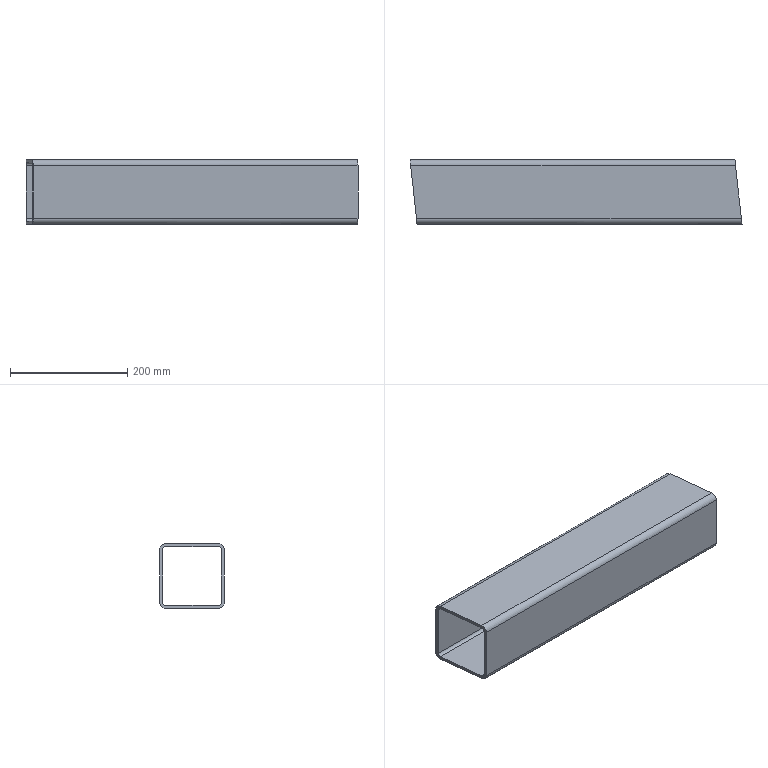Part | SolidWorks | features 3DProfileFeature 1, ICE 1, WeldMemberFeat 1, WeldmentFeature 1 | 1 solid | 18 faces | box 565.469 x 110 x 110 mm | volume 1126381 mm3 | plane 10 | cylinder 8 | commonest cylinder face diameters 10 x4 20 x4
STEP:
#1=CARTESIAN_POINT('',(563.658,55.,-45.));
#2=VERTEX_POINT('',#1);
#3=CARTESIAN_POINT('',(10.323,55.,-45.));
#4=VERTEX_POINT('',#3);
#5=CARTESIAN_POINT('',(600.,55.,-45.));
#6=DIRECTION('',(-1.,0.,0.));
#7=VECTOR('',#6,1000.);
#8=LINE('',#5,#7);
#9=EDGE_CURVE('',#2,#4,#8,.T.);
#10=ORIENTED_EDGE('',*,*,#9,.F.);
#11=CARTESIAN_POINT('',(564.761,45.,-55.));
#12=VERTEX_POINT('',#11);
#13=CARTESIAN_POINT('',(563.658,55.,-45.));
#14=CARTESIAN_POINT('',(563.658,55.,-50.858));
#15=CARTESIAN_POINT('',(564.115,50.858,-55.));
#16=CARTESIAN_POINT('',(564.761,45.,-55.));
#17=(BOUNDED_CURVE()B_SPLINE_CURVE(3,(#13,#14,#15,#16),.UNSPECIFIED.,.F.,.F.)B_SPLINE_CURVE_WITH_KNOTS((4,4),(0.,1.571),.UNSPECIFIED.)CURVE()GEOMETRIC_REPRESENTATION_ITEM()RATIONAL_B_SPLINE_CURVE((1.,0.8047,0.8047,1.))REPRESENTATION_ITEM(''));
#18=EDGE_CURVE('',#2,#12,#17,.T.);
#19=ORIENTED_EDGE('',*,*,#18,.T.);
#20=CARTESIAN_POINT('',(11.426,45.,-55.));
#21=VERTEX_POINT('',#20);
#22=CARTESIAN_POINT('',(600.,45.,-55.));
#23=DIRECTION('',(-1.,0.,0.));
#24=VECTOR('',#23,1000.);
#25=LINE('',#22,#24);
#26=EDGE_CURVE('',#12,#21,#25,.T.);
#27=ORIENTED_EDGE('',*,*,#26,.T.);
#28=CARTESIAN_POINT('',(11.426,45.,-55.));
#29=CARTESIAN_POINT('',(10.779,50.858,-55.));
#30=CARTESIAN_POINT('',(10.323,55.,-50.858));
#31=CARTESIAN_POINT('',(10.323,55.,-45.));
#32=(BOUNDED_CURVE()B_SPLINE_CURVE(3,(#28,#29,#30,#31),.UNSPECIFIED.,.F.,.F.)B_SPLINE_CURVE_WITH_KNOTS((4,4),(4.712,6.283),.UNSPECIFIED.)CURVE()GEOMETRIC_REPRESENTATION_ITEM()RATIONAL_B_SPLINE_CURVE((1.,0.8047,0.8047,1.))REPRESENTATION_ITEM(''));
#33=EDGE_CURVE('',#21,#4,#32,.T.);
#34=ORIENTED_EDGE('',*,*,#33,.T.);
#35=EDGE_LOOP('',(#10,#19,#27,#34));
#36=FACE_OUTER_BOUND('',#35,.T.);
#37=CARTESIAN_POINT('',(600.,45.,-45.));
#38=DIRECTION('',(-1.,0.,0.));
#39=DIRECTION('',(0.,0.,1.));
#40=AXIS2_PLACEMENT_3D('',#37,#38,#39);
#41=CYLINDRICAL_SURFACE('',#40,10.);
#42=ADVANCED_FACE('',(#36),#41,.T.);
#43=CARTESIAN_POINT('',(563.658,55.,45.));
#44=VERTEX_POINT('',#43);
#45=CARTESIAN_POINT('',(10.323,55.,45.));
#46=VERTEX_POINT('',#45);
#47=CARTESIAN_POINT('',(600.,55.,45.));
#48=DIRECTION('',(-1.,0.,0.));
#49=VECTOR('',#48,1000.);
#50=LINE('',#47,#49);
#51=EDGE_CURVE('',#44,#46,#50,.T.);
#52=ORIENTED_EDGE('',*,*,#51,.F.);
#53=CARTESIAN_POINT('',(563.658,55.,-386.466));
#54=DIRECTION('',(0.,0.,1.));
#55=VECTOR('',#54,1000.);
#56=LINE('',#53,#55);
#57=EDGE_CURVE('',#2,#44,#56,.T.);
#58=ORIENTED_EDGE('',*,*,#57,.F.);
#59=ORIENTED_EDGE('',*,*,#9,.T.);
#60=CARTESIAN_POINT('',(10.323,55.,-45.));
#61=DIRECTION('',(0.,0.,1.));
#62=VECTOR('',#61,1000.);
#63=LINE('',#60,#62);
#64=EDGE_CURVE('',#4,#46,#63,.T.);
#65=ORIENTED_EDGE('',*,*,#64,.T.);
#66=EDGE_LOOP('',(#52,#58,#59,#65));
#67=FACE_OUTER_BOUND('',#66,.T.);
#68=CARTESIAN_POINT('',(600.,55.,-45.));
#69=DIRECTION('',(0.,-1.,0.));
#70=DIRECTION('',(0.,0.,-1.));
#71=AXIS2_PLACEMENT_3D('',#68,#69,#70);
#72=PLANE('',#71);
#73=ADVANCED_FACE('',(#67),#72,.F.);
#74=CARTESIAN_POINT('',(564.761,45.,55.));
#75=VERTEX_POINT('',#74);
#76=CARTESIAN_POINT('',(11.426,45.,55.));
#77=VERTEX_POINT('',#76);
#78=CARTESIAN_POINT('',(600.,45.,55.));
#79=DIRECTION('',(-1.,0.,0.));
#80=VECTOR('',#79,1000.);
#81=LINE('',#78,#80);
#82=EDGE_CURVE('',#75,#77,#81,.T.);
#83=ORIENTED_EDGE('',*,*,#82,.F.);
#84=CARTESIAN_POINT('',(564.761,45.,55.));
#85=CARTESIAN_POINT('',(564.115,50.858,55.));
#86=CARTESIAN_POINT('',(563.658,55.,50.858));
#87=CARTESIAN_POINT('',(563.658,55.,45.));
#88=(BOUNDED_CURVE()B_SPLINE_CURVE(3,(#84,#85,#86,#87),.UNSPECIFIED.,.F.,.F.)B_SPLINE_CURVE_WITH_KNOTS((4,4),(4.712,6.283),.UNSPECIFIED.)CURVE()GEOMETRIC_REPRESENTATION_ITEM()RATIONAL_B_SPLINE_CURVE((1.,0.8047,0.8047,1.))REPRESENTATION_ITEM(''));
#89=EDGE_CURVE('',#75,#44,#88,.T.);
#90=ORIENTED_EDGE('',*,*,#89,.T.);
#91=ORIENTED_EDGE('',*,*,#51,.T.);
#92=CARTESIAN_POINT('',(10.323,55.,45.));
#93=CARTESIAN_POINT('',(10.323,55.,50.858));
#94=CARTESIAN_POINT('',(10.779,50.858,55.));
#95=CARTESIAN_POINT('',(11.426,45.,55.));
#96=(BOUNDED_CURVE()B_SPLINE_CURVE(3,(#92,#93,#94,#95),.UNSPECIFIED.,.F.,.F.)B_SPLINE_CURVE_WITH_KNOTS((4,4),(0.,1.571),.UNSPECIFIED.)CURVE()GEOMETRIC_REPRESENTATION_ITEM()RATIONAL_B_SPLINE_CURVE((1.,0.8047,0.8047,1.))REPRESENTATION_ITEM(''));
#97=EDGE_CURVE('',#46,#77,#96,.T.);
#98=ORIENTED_EDGE('',*,*,#97,.T.);
#99=EDGE_LOOP('',(#83,#90,#91,#98));
#100=FACE_OUTER_BOUND('',#99,.T.);
#101=CARTESIAN_POINT('',(600.,45.,45.));
#102=DIRECTION('',(-1.,0.,0.));
#103=DIRECTION('',(0.,0.,1.));
#104=AXIS2_PLACEMENT_3D('',#101,#102,#103);
#105=CYLINDRICAL_SURFACE('',#104,10.);
#106=ADVANCED_FACE('',(#100),#105,.T.);
#107=CARTESIAN_POINT('',(574.689,-45.,55.));
#108=VERTEX_POINT('',#107);
#109=CARTESIAN_POINT('',(21.353,-45.,55.));
#110=VERTEX_POINT('',#109);
#111=CARTESIAN_POINT('',(600.,-45.,55.));
#112=DIRECTION('',(-1.,0.,0.));
#113=VECTOR('',#112,1000.);
#114=LINE('',#111,#113);
#115=EDGE_CURVE('',#108,#110,#114,.T.);
#116=ORIENTED_EDGE('',*,*,#115,.F.);
#117=CARTESIAN_POINT('',(600.,-274.468,55.));
#118=DIRECTION('',(0.1096,-0.994,0.));
#119=VECTOR('',#118,1000.);
#120=LINE('',#117,#119);
#121=EDGE_CURVE('',#75,#108,#120,.T.);
#122=ORIENTED_EDGE('',*,*,#121,.F.);
#123=ORIENTED_EDGE('',*,*,#82,.T.);
#124=CARTESIAN_POINT('',(0.,148.583,55.));
#125=DIRECTION('',(-0.1096,0.994,0.));
#126=VECTOR('',#125,1000.);
#127=LINE('',#124,#126);
#128=EDGE_CURVE('',#110,#77,#127,.T.);
#129=ORIENTED_EDGE('',*,*,#128,.F.);
#130=EDGE_LOOP('',(#116,#122,#123,#129));
#131=FACE_OUTER_BOUND('',#130,.T.);
#132=CARTESIAN_POINT('',(600.,-45.,55.));
#133=DIRECTION('',(0.,0.,-1.));
#134=DIRECTION('',(-1.,0.,0.));
#135=AXIS2_PLACEMENT_3D('',#132,#133,#134);
#136=PLANE('',#135);
#137=ADVANCED_FACE('',(#131),#136,.F.);
#138=CARTESIAN_POINT('',(575.792,-55.,45.));
#139=VERTEX_POINT('',#138);
#140=CARTESIAN_POINT('',(22.456,-55.,45.));
#141=VERTEX_POINT('',#140);
#142=CARTESIAN_POINT('',(600.,-55.,45.));
#143=DIRECTION('',(-1.,0.,0.));
#144=VECTOR('',#143,1000.);
#145=LINE('',#142,#144);
#146=EDGE_CURVE('',#139,#141,#145,.T.);
#147=ORIENTED_EDGE('',*,*,#146,.F.);
#148=CARTESIAN_POINT('',(575.792,-55.,45.));
#149=CARTESIAN_POINT('',(575.792,-55.,50.858));
#150=CARTESIAN_POINT('',(575.335,-50.858,55.));
#151=CARTESIAN_POINT('',(574.689,-45.,55.));
#152=(BOUNDED_CURVE()B_SPLINE_CURVE(3,(#148,#149,#150,#151),.UNSPECIFIED.,.F.,.F.)B_SPLINE_CURVE_WITH_KNOTS((4,4),(3.142,4.712),.UNSPECIFIED.)CURVE()GEOMETRIC_REPRESENTATION_ITEM()RATIONAL_B_SPLINE_CURVE((1.,0.8047,0.8047,1.))REPRESENTATION_ITEM(''));
#153=EDGE_CURVE('',#139,#108,#152,.T.);
#154=ORIENTED_EDGE('',*,*,#153,.T.);
#155=ORIENTED_EDGE('',*,*,#115,.T.);
#156=CARTESIAN_POINT('',(21.353,-45.,55.));
#157=CARTESIAN_POINT('',(21.999,-50.858,55.));
#158=CARTESIAN_POINT('',(22.456,-55.,50.858));
#159=CARTESIAN_POINT('',(22.456,-55.,45.));
#160=(BOUNDED_CURVE()B_SPLINE_CURVE(3,(#156,#157,#158,#159),.UNSPECIFIED.,.F.,.F.)B_SPLINE_CURVE_WITH_KNOTS((4,4),(1.571,3.142),.UNSPECIFIED.)CURVE()GEOMETRIC_REPRESENTATION_ITEM()RATIONAL_B_SPLINE_CURVE((1.,0.8047,0.8047,1.))REPRESENTATION_ITEM(''));
#161=EDGE_CURVE('',#110,#141,#160,.T.);
#162=ORIENTED_EDGE('',*,*,#161,.T.);
#163=EDGE_LOOP('',(#147,#154,#155,#162));
#164=FACE_OUTER_BOUND('',#163,.T.);
#165=CARTESIAN_POINT('',(600.,-45.,45.));
#166=DIRECTION('',(-1.,0.,0.));
#167=DIRECTION('',(0.,0.,1.));
#168=AXIS2_PLACEMENT_3D('',#165,#166,#167);
#169=CYLINDRICAL_SURFACE('',#168,10.);
#170=ADVANCED_FACE('',(#164),#169,.T.);
#171=CARTESIAN_POINT('',(575.792,-55.,-45.));
#172=VERTEX_POINT('',#171);
#173=CARTESIAN_POINT('',(22.456,-55.,-45.));
#174=VERTEX_POINT('',#173);
#175=CARTESIAN_POINT('',(600.,-55.,-45.));
#176=DIRECTION('',(-1.,0.,0.));
#177=VECTOR('',#176,1000.);
#178=LINE('',#175,#177);
#179=EDGE_CURVE('',#172,#174,#178,.T.);
#180=ORIENTED_EDGE('',*,*,#179,.F.);
#181=CARTESIAN_POINT('',(575.792,-55.,45.));
#182=DIRECTION('',(0.,0.,1.));
#183=VECTOR('',#182,1000.);
#184=LINE('',#181,#183);
#185=EDGE_CURVE('',#172,#139,#184,.T.);
#186=ORIENTED_EDGE('',*,*,#185,.T.);
#187=ORIENTED_EDGE('',*,*,#146,.T.);
#188=CARTESIAN_POINT('',(22.456,-55.,-386.466));
#189=DIRECTION('',(0.,0.,1.));
#190=VECTOR('',#189,1000.);
#191=LINE('',#188,#190);
#192=EDGE_CURVE('',#174,#141,#191,.T.);
#193=ORIENTED_EDGE('',*,*,#192,.F.);
#194=EDGE_LOOP('',(#180,#186,#187,#193));
#195=FACE_OUTER_BOUND('',#194,.T.);
#196=CARTESIAN_POINT('',(600.,-55.,45.));
#197=DIRECTION('',(0.,1.,0.));
#198=DIRECTION('',(0.,0.,1.));
#199=AXIS2_PLACEMENT_3D('',#196,#197,#198);
#200=PLANE('',#199);
#201=ADVANCED_FACE('',(#195),#200,.F.);
#202=CARTESIAN_POINT('',(574.689,-45.,-55.));
#203=VERTEX_POINT('',#202);
#204=CARTESIAN_POINT('',(21.353,-45.,-55.));
#205=VERTEX_POINT('',#204);
#206=CARTESIAN_POINT('',(600.,-45.,-55.));
#207=DIRECTION('',(-1.,0.,0.));
#208=VECTOR('',#207,1000.);
#209=LINE('',#206,#208);
#210=EDGE_CURVE('',#203,#205,#209,.T.);
#211=ORIENTED_EDGE('',*,*,#210,.F.);
#212=CARTESIAN_POINT('',(574.689,-45.,-55.));
#213=CARTESIAN_POINT('',(575.335,-50.858,-55.));
#214=CARTESIAN_POINT('',(575.792,-55.,-50.858));
#215=CARTESIAN_POINT('',(575.792,-55.,-45.));
#216=(BOUNDED_CURVE()B_SPLINE_CURVE(3,(#212,#213,#214,#215),.UNSPECIFIED.,.F.,.F.)B_SPLINE_CURVE_WITH_KNOTS((4,4),(1.571,3.142),.UNSPECIFIED.)CURVE()GEOMETRIC_REPRESENTATION_ITEM()RATIONAL_B_SPLINE_CURVE((1.,0.8047,0.8047,1.))REPRESENTATION_ITEM(''));
#217=EDGE_CURVE('',#203,#172,#216,.T.);
#218=ORIENTED_EDGE('',*,*,#217,.T.);
#219=ORIENTED_EDGE('',*,*,#179,.T.);
#220=CARTESIAN_POINT('',(22.456,-55.,-45.));
#221=CARTESIAN_POINT('',(22.456,-55.,-50.858));
#222=CARTESIAN_POINT('',(21.999,-50.858,-55.));
#223=CARTESIAN_POINT('',(21.353,-45.,-55.));
#224=(BOUNDED_CURVE()B_SPLINE_CURVE(3,(#220,#221,#222,#223),.UNSPECIFIED.,.F.,.F.)B_SPLINE_CURVE_WITH_KNOTS((4,4),(3.142,4.712),.UNSPECIFIED.)CURVE()GEOMETRIC_REPRESENTATION_ITEM()RATIONAL_B_SPLINE_CURVE((1.,0.8047,0.8047,1.))REPRESENTATION_ITEM(''));
#225=EDGE_CURVE('',#174,#205,#224,.T.);
#226=ORIENTED_EDGE('',*,*,#225,.T.);
#227=EDGE_LOOP('',(#211,#218,#219,#226));
#228=FACE_OUTER_BOUND('',#227,.T.);
#229=CARTESIAN_POINT('',(600.,-45.,-45.));
#230=DIRECTION('',(-1.,0.,0.));
#231=DIRECTION('',(0.,0.,1.));
#232=AXIS2_PLACEMENT_3D('',#229,#230,#231);
#233=CYLINDRICAL_SURFACE('',#232,10.);
#234=ADVANCED_FACE('',(#228),#233,.T.);
#235=CARTESIAN_POINT('',(564.761,45.,50.));
#236=VERTEX_POINT('',#235);
#237=CARTESIAN_POINT('',(564.21,50.,45.));
#238=VERTEX_POINT('',#237);
#239=CARTESIAN_POINT('',(564.761,45.,50.));
#240=CARTESIAN_POINT('',(564.438,47.929,50.));
#241=CARTESIAN_POINT('',(564.21,50.,47.929));
#242=CARTESIAN_POINT('',(564.21,50.,45.));
#243=(BOUNDED_CURVE()B_SPLINE_CURVE(3,(#239,#240,#241,#242),.UNSPECIFIED.,.F.,.F.)B_SPLINE_CURVE_WITH_KNOTS((4,4),(4.712,6.283),.UNSPECIFIED.)CURVE()GEOMETRIC_REPRESENTATION_ITEM()RATIONAL_B_SPLINE_CURVE((1.,0.8047,0.8047,1.))REPRESENTATION_ITEM(''));
#244=EDGE_CURVE('',#236,#238,#243,.T.);
#245=ORIENTED_EDGE('',*,*,#244,.F.);
#246=CARTESIAN_POINT('',(11.426,45.,50.));
#247=VERTEX_POINT('',#246);
#248=CARTESIAN_POINT('',(600.,45.,50.));
#249=DIRECTION('',(-1.,0.,0.));
#250=VECTOR('',#249,1000.);
#251=LINE('',#248,#250);
#252=EDGE_CURVE('',#236,#247,#251,.T.);
#253=ORIENTED_EDGE('',*,*,#252,.T.);
#254=CARTESIAN_POINT('',(10.874,50.,45.));
#255=VERTEX_POINT('',#254);
#256=CARTESIAN_POINT('',(10.874,50.,45.));
#257=CARTESIAN_POINT('',(10.874,50.,47.929));
#258=CARTESIAN_POINT('',(11.103,47.929,50.));
#259=CARTESIAN_POINT('',(11.426,45.,50.));
#260=(BOUNDED_CURVE()B_SPLINE_CURVE(3,(#256,#257,#258,#259),.UNSPECIFIED.,.F.,.F.)B_SPLINE_CURVE_WITH_KNOTS((4,4),(0.,1.571),.UNSPECIFIED.)CURVE()GEOMETRIC_REPRESENTATION_ITEM()RATIONAL_B_SPLINE_CURVE((1.,0.8047,0.8047,1.))REPRESENTATION_ITEM(''));
#261=EDGE_CURVE('',#255,#247,#260,.T.);
#262=ORIENTED_EDGE('',*,*,#261,.F.);
#263=CARTESIAN_POINT('',(600.,50.,45.));
#264=DIRECTION('',(-1.,0.,0.));
#265=VECTOR('',#264,1000.);
#266=LINE('',#263,#265);
#267=EDGE_CURVE('',#238,#255,#266,.T.);
#268=ORIENTED_EDGE('',*,*,#267,.F.);
#269=EDGE_LOOP('',(#245,#253,#262,#268));
#270=FACE_OUTER_BOUND('',#269,.T.);
#271=CARTESIAN_POINT('',(600.,45.,45.));
#272=DIRECTION('',(-1.,0.,0.));
#273=DIRECTION('',(0.,0.,1.));
#274=AXIS2_PLACEMENT_3D('',#271,#272,#273);
#275=CYLINDRICAL_SURFACE('',#274,5.);
#276=ADVANCED_FACE('',(#270),#275,.F.);
#277=CARTESIAN_POINT('',(564.21,50.,-45.));
#278=VERTEX_POINT('',#277);
#279=CARTESIAN_POINT('',(564.21,50.,-45.));
#280=DIRECTION('',(0.,0.,-1.));
#281=VECTOR('',#280,1000.);
#282=LINE('',#279,#281);
#283=EDGE_CURVE('',#238,#278,#282,.T.);
#284=ORIENTED_EDGE('',*,*,#283,.F.);
#285=ORIENTED_EDGE('',*,*,#267,.T.);
#286=CARTESIAN_POINT('',(10.874,50.,-45.));
#287=VERTEX_POINT('',#286);
#288=CARTESIAN_POINT('',(10.874,50.,-45.));
#289=DIRECTION('',(0.,0.,1.));
#290=VECTOR('',#289,1000.);
#291=LINE('',#288,#290);
#292=EDGE_CURVE('',#287,#255,#291,.T.);
#293=ORIENTED_EDGE('',*,*,#292,.F.);
#294=CARTESIAN_POINT('',(600.,50.,-45.));
#295=DIRECTION('',(-1.,0.,0.));
#296=VECTOR('',#295,1000.);
#297=LINE('',#294,#296);
#298=EDGE_CURVE('',#278,#287,#297,.T.);
#299=ORIENTED_EDGE('',*,*,#298,.F.);
#300=EDGE_LOOP('',(#284,#285,#293,#299));
#301=FACE_OUTER_BOUND('',#300,.T.);
#302=CARTESIAN_POINT('',(600.,50.,-45.));
#303=DIRECTION('',(0.,-1.,0.));
#304=DIRECTION('',(0.,0.,-1.));
#305=AXIS2_PLACEMENT_3D('',#302,#303,#304);
#306=PLANE('',#305);
#307=ADVANCED_FACE('',(#301),#306,.T.);
#308=CARTESIAN_POINT('',(564.761,45.,-50.));
#309=VERTEX_POINT('',#308);
#310=CARTESIAN_POINT('',(564.21,50.,-45.));
#311=CARTESIAN_POINT('',(564.21,50.,-47.929));
#312=CARTESIAN_POINT('',(564.438,47.929,-50.));
#313=CARTESIAN_POINT('',(564.761,45.,-50.));
#314=(BOUNDED_CURVE()B_SPLINE_CURVE(3,(#310,#311,#312,#313),.UNSPECIFIED.,.F.,.F.)B_SPLINE_CURVE_WITH_KNOTS((4,4),(0.,1.571),.UNSPECIFIED.)CURVE()GEOMETRIC_REPRESENTATION_ITEM()RATIONAL_B_SPLINE_CURVE((1.,0.8047,0.8047,1.))REPRESENTATION_ITEM(''));
#315=EDGE_CURVE('',#278,#309,#314,.T.);
#316=ORIENTED_EDGE('',*,*,#315,.F.);
#317=ORIENTED_EDGE('',*,*,#298,.T.);
#318=CARTESIAN_POINT('',(11.426,45.,-50.));
#319=VERTEX_POINT('',#318);
#320=CARTESIAN_POINT('',(11.426,45.,-50.));
#321=CARTESIAN_POINT('',(11.103,47.929,-50.));
#322=CARTESIAN_POINT('',(10.874,50.,-47.929));
#323=CARTESIAN_POINT('',(10.874,50.,-45.));
#324=(BOUNDED_CURVE()B_SPLINE_CURVE(3,(#320,#321,#322,#323),.UNSPECIFIED.,.F.,.F.)B_SPLINE_CURVE_WITH_KNOTS((4,4),(4.712,6.283),.UNSPECIFIED.)CURVE()GEOMETRIC_REPRESENTATION_ITEM()RATIONAL_B_SPLINE_CURVE((1.,0.8047,0.8047,1.))REPRESENTATION_ITEM(''));
#325=EDGE_CURVE('',#319,#287,#324,.T.);
#326=ORIENTED_EDGE('',*,*,#325,.F.);
#327=CARTESIAN_POINT('',(600.,45.,-50.));
#328=DIRECTION('',(-1.,0.,0.));
#329=VECTOR('',#328,1000.);
#330=LINE('',#327,#329);
#331=EDGE_CURVE('',#309,#319,#330,.T.);
#332=ORIENTED_EDGE('',*,*,#331,.F.);
#333=EDGE_LOOP('',(#316,#317,#326,#332));
#334=FACE_OUTER_BOUND('',#333,.T.);
#335=CARTESIAN_POINT('',(600.,45.,-45.));
#336=DIRECTION('',(-1.,0.,0.));
#337=DIRECTION('',(0.,0.,1.));
#338=AXIS2_PLACEMENT_3D('',#335,#336,#337);
#339=CYLINDRICAL_SURFACE('',#338,5.);
#340=ADVANCED_FACE('',(#334),#339,.F.);
#341=CARTESIAN_POINT('',(574.689,-45.,-50.));
#342=VERTEX_POINT('',#341);
#343=CARTESIAN_POINT('',(565.185,41.16,-50.));
#344=DIRECTION('',(0.1096,-0.994,0.));
#345=VECTOR('',#344,1000.);
#346=LINE('',#343,#345);
#347=EDGE_CURVE('',#309,#342,#346,.T.);
#348=ORIENTED_EDGE('',*,*,#347,.F.);
#349=ORIENTED_EDGE('',*,*,#331,.T.);
#350=CARTESIAN_POINT('',(21.353,-45.,-50.));
#351=VERTEX_POINT('',#350);
#352=CARTESIAN_POINT('',(18.501,-19.142,-50.));
#353=DIRECTION('',(-0.1096,0.994,0.));
#354=VECTOR('',#353,1000.);
#355=LINE('',#352,#354);
#356=EDGE_CURVE('',#351,#319,#355,.T.);
#357=ORIENTED_EDGE('',*,*,#356,.F.);
#358=CARTESIAN_POINT('',(600.,-45.,-50.));
#359=DIRECTION('',(-1.,0.,0.));
#360=VECTOR('',#359,1000.);
#361=LINE('',#358,#360);
#362=EDGE_CURVE('',#342,#351,#361,.T.);
#363=ORIENTED_EDGE('',*,*,#362,.F.);
#364=EDGE_LOOP('',(#348,#349,#357,#363));
#365=FACE_OUTER_BOUND('',#364,.T.);
#366=CARTESIAN_POINT('',(600.,45.,-50.));
#367=DIRECTION('',(0.,0.,1.));
#368=DIRECTION('',(1.,0.,0.));
#369=AXIS2_PLACEMENT_3D('',#366,#367,#368);
#370=PLANE('',#369);
#371=ADVANCED_FACE('',(#365),#370,.T.);
#372=CARTESIAN_POINT('',(575.24,-50.,-45.));
#373=VERTEX_POINT('',#372);
#374=CARTESIAN_POINT('',(574.689,-45.,-50.));
#375=CARTESIAN_POINT('',(575.012,-47.929,-50.));
#376=CARTESIAN_POINT('',(575.24,-50.,-47.929));
#377=CARTESIAN_POINT('',(575.24,-50.,-45.));
#378=(BOUNDED_CURVE()B_SPLINE_CURVE(3,(#374,#375,#376,#377),.UNSPECIFIED.,.F.,.F.)B_SPLINE_CURVE_WITH_KNOTS((4,4),(1.571,3.142),.UNSPECIFIED.)CURVE()GEOMETRIC_REPRESENTATION_ITEM()RATIONAL_B_SPLINE_CURVE((1.,0.8047,0.8047,1.))REPRESENTATION_ITEM(''));
#379=EDGE_CURVE('',#342,#373,#378,.T.);
#380=ORIENTED_EDGE('',*,*,#379,.F.);
#381=ORIENTED_EDGE('',*,*,#362,.T.);
#382=CARTESIAN_POINT('',(21.904,-50.,-45.));
#383=VERTEX_POINT('',#382);
#384=CARTESIAN_POINT('',(21.904,-50.,-45.));
#385=CARTESIAN_POINT('',(21.904,-50.,-47.929));
#386=CARTESIAN_POINT('',(21.676,-47.929,-50.));
#387=CARTESIAN_POINT('',(21.353,-45.,-50.));
#388=(BOUNDED_CURVE()B_SPLINE_CURVE(3,(#384,#385,#386,#387),.UNSPECIFIED.,.F.,.F.)B_SPLINE_CURVE_WITH_KNOTS((4,4),(3.142,4.712),.UNSPECIFIED.)CURVE()GEOMETRIC_REPRESENTATION_ITEM()RATIONAL_B_SPLINE_CURVE((1.,0.8047,0.8047,1.))REPRESENTATION_ITEM(''));
#389=EDGE_CURVE('',#383,#351,#388,.T.);
#390=ORIENTED_EDGE('',*,*,#389,.F.);
#391=CARTESIAN_POINT('',(600.,-50.,-45.));
#392=DIRECTION('',(-1.,0.,0.));
#393=VECTOR('',#392,1000.);
#394=LINE('',#391,#393);
#395=EDGE_CURVE('',#373,#383,#394,.T.);
#396=ORIENTED_EDGE('',*,*,#395,.F.);
#397=EDGE_LOOP('',(#380,#381,#390,#396));
#398=FACE_OUTER_BOUND('',#397,.T.);
#399=CARTESIAN_POINT('',(600.,-45.,-45.));
#400=DIRECTION('',(-1.,0.,0.));
#401=DIRECTION('',(0.,0.,1.));
#402=AXIS2_PLACEMENT_3D('',#399,#400,#401);
#403=CYLINDRICAL_SURFACE('',#402,5.);
#404=ADVANCED_FACE('',(#398),#403,.F.);
#405=CARTESIAN_POINT('',(575.24,-50.,45.));
#406=VERTEX_POINT('',#405);
#407=CARTESIAN_POINT('',(575.24,-50.,45.));
#408=DIRECTION('',(0.,0.,1.));
#409=VECTOR('',#408,1000.);
#410=LINE('',#407,#409);
#411=EDGE_CURVE('',#373,#406,#410,.T.);
#412=ORIENTED_EDGE('',*,*,#411,.F.);
#413=ORIENTED_EDGE('',*,*,#395,.T.);
#414=CARTESIAN_POINT('',(21.904,-50.,45.));
#415=VERTEX_POINT('',#414);
#416=CARTESIAN_POINT('',(21.904,-50.,45.));
#417=DIRECTION('',(0.,0.,-1.));
#418=VECTOR('',#417,1000.);
#419=LINE('',#416,#418);
#420=EDGE_CURVE('',#415,#383,#419,.T.);
#421=ORIENTED_EDGE('',*,*,#420,.F.);
#422=CARTESIAN_POINT('',(600.,-50.,45.));
#423=DIRECTION('',(-1.,0.,0.));
#424=VECTOR('',#423,1000.);
#425=LINE('',#422,#424);
#426=EDGE_CURVE('',#406,#415,#425,.T.);
#427=ORIENTED_EDGE('',*,*,#426,.F.);
#428=EDGE_LOOP('',(#412,#413,#421,#427));
#429=FACE_OUTER_BOUND('',#428,.T.);
#430=CARTESIAN_POINT('',(600.,-50.,45.));
#431=DIRECTION('',(0.,1.,0.));
#432=DIRECTION('',(0.,0.,1.));
#433=AXIS2_PLACEMENT_3D('',#430,#431,#432);
#434=PLANE('',#433);
#435=ADVANCED_FACE('',(#429),#434,.T.);
#436=CARTESIAN_POINT('',(574.689,-45.,50.));
#437=VERTEX_POINT('',#436);
#438=CARTESIAN_POINT('',(575.24,-50.,45.));
#439=CARTESIAN_POINT('',(575.24,-50.,47.929));
#440=CARTESIAN_POINT('',(575.012,-47.929,50.));
#441=CARTESIAN_POINT('',(574.689,-45.,50.));
#442=(BOUNDED_CURVE()B_SPLINE_CURVE(3,(#438,#439,#440,#441),.UNSPECIFIED.,.F.,.F.)B_SPLINE_CURVE_WITH_KNOTS((4,4),(3.142,4.712),.UNSPECIFIED.)CURVE()GEOMETRIC_REPRESENTATION_ITEM()RATIONAL_B_SPLINE_CURVE((1.,0.8047,0.8047,1.))REPRESENTATION_ITEM(''));
#443=EDGE_CURVE('',#406,#437,#442,.T.);
#444=ORIENTED_EDGE('',*,*,#443,.F.);
#445=ORIENTED_EDGE('',*,*,#426,.T.);
#446=CARTESIAN_POINT('',(21.353,-45.,50.));
#447=VERTEX_POINT('',#446);
#448=CARTESIAN_POINT('',(21.353,-45.,50.));
#449=CARTESIAN_POINT('',(21.676,-47.929,50.));
#450=CARTESIAN_POINT('',(21.904,-50.,47.929));
#451=CARTESIAN_POINT('',(21.904,-50.,45.));
#452=(BOUNDED_CURVE()B_SPLINE_CURVE(3,(#448,#449,#450,#451),.UNSPECIFIED.,.F.,.F.)B_SPLINE_CURVE_WITH_KNOTS((4,4),(1.571,3.142),.UNSPECIFIED.)CURVE()GEOMETRIC_REPRESENTATION_ITEM()RATIONAL_B_SPLINE_CURVE((1.,0.8047,0.8047,1.))REPRESENTATION_ITEM(''));
#453=EDGE_CURVE('',#447,#415,#452,.T.);
#454=ORIENTED_EDGE('',*,*,#453,.F.);
#455=CARTESIAN_POINT('',(600.,-45.,50.));
#456=DIRECTION('',(-1.,0.,0.));
#457=VECTOR('',#456,1000.);
#458=LINE('',#455,#457);
#459=EDGE_CURVE('',#437,#447,#458,.T.);
#460=ORIENTED_EDGE('',*,*,#459,.F.);
#461=EDGE_LOOP('',(#444,#445,#454,#460));
#462=FACE_OUTER_BOUND('',#461,.T.);
#463=CARTESIAN_POINT('',(600.,-45.,45.));
#464=DIRECTION('',(-1.,0.,0.));
#465=DIRECTION('',(0.,0.,1.));
#466=AXIS2_PLACEMENT_3D('',#463,#464,#465);
#467=CYLINDRICAL_SURFACE('',#466,5.);
#468=ADVANCED_FACE('',(#462),#467,.F.);
#469=CARTESIAN_POINT('',(574.993,-47.758,50.));
#470=DIRECTION('',(-0.1096,0.994,0.));
#471=VECTOR('',#470,1000.);
#472=LINE('',#469,#471);
#473=EDGE_CURVE('',#437,#236,#472,.T.);
#474=ORIENTED_EDGE('',*,*,#473,.F.);
#475=ORIENTED_EDGE('',*,*,#459,.T.);
#476=CARTESIAN_POINT('',(28.309,-108.06,50.));
#477=DIRECTION('',(0.1096,-0.994,0.));
#478=VECTOR('',#477,1000.);
#479=LINE('',#476,#478);
#480=EDGE_CURVE('',#247,#447,#479,.T.);
#481=ORIENTED_EDGE('',*,*,#480,.F.);
#482=ORIENTED_EDGE('',*,*,#252,.F.);
#483=EDGE_LOOP('',(#474,#475,#481,#482));
#484=FACE_OUTER_BOUND('',#483,.T.);
#485=CARTESIAN_POINT('',(600.,-45.,50.));
#486=DIRECTION('',(0.,0.,-1.));
#487=DIRECTION('',(-1.,0.,0.));
#488=AXIS2_PLACEMENT_3D('',#485,#486,#487);
#489=PLANE('',#488);
#490=ADVANCED_FACE('',(#484),#489,.T.);
#491=ORIENTED_EDGE('',*,*,#26,.F.);
#492=CARTESIAN_POINT('',(600.,-274.468,-55.));
#493=DIRECTION('',(-0.1096,0.994,0.));
#494=VECTOR('',#493,1000.);
#495=LINE('',#492,#494);
#496=EDGE_CURVE('',#203,#12,#495,.T.);
#497=ORIENTED_EDGE('',*,*,#496,.F.);
#498=ORIENTED_EDGE('',*,*,#210,.T.);
#499=CARTESIAN_POINT('',(0.,148.583,-55.));
#500=DIRECTION('',(0.1096,-0.994,0.));
#501=VECTOR('',#500,1000.);
#502=LINE('',#499,#501);
#503=EDGE_CURVE('',#21,#205,#502,.T.);
#504=ORIENTED_EDGE('',*,*,#503,.F.);
#505=EDGE_LOOP('',(#491,#497,#498,#504));
#506=FACE_OUTER_BOUND('',#505,.T.);
#507=CARTESIAN_POINT('',(600.,45.,-55.));
#508=DIRECTION('',(0.,0.,1.));
#509=DIRECTION('',(1.,0.,0.));
#510=AXIS2_PLACEMENT_3D('',#507,#508,#509);
#511=PLANE('',#510);
#512=ADVANCED_FACE('',(#506),#511,.F.);
#513=ORIENTED_EDGE('',*,*,#261,.T.);
#514=ORIENTED_EDGE('',*,*,#480,.T.);
#515=ORIENTED_EDGE('',*,*,#453,.T.);
#516=ORIENTED_EDGE('',*,*,#420,.T.);
#517=ORIENTED_EDGE('',*,*,#389,.T.);
#518=ORIENTED_EDGE('',*,*,#356,.T.);
#519=ORIENTED_EDGE('',*,*,#325,.T.);
#520=ORIENTED_EDGE('',*,*,#292,.T.);
#521=EDGE_LOOP('',(#513,#514,#515,#516,#517,#518,#519,#520));
#522=FACE_BOUND('',#521,.T.);
#523=ORIENTED_EDGE('',*,*,#503,.T.);
#524=ORIENTED_EDGE('',*,*,#225,.F.);
#525=ORIENTED_EDGE('',*,*,#192,.T.);
#526=ORIENTED_EDGE('',*,*,#161,.F.);
#527=ORIENTED_EDGE('',*,*,#128,.T.);
#528=ORIENTED_EDGE('',*,*,#97,.F.);
#529=ORIENTED_EDGE('',*,*,#64,.F.);
#530=ORIENTED_EDGE('',*,*,#33,.F.);
#531=EDGE_LOOP('',(#523,#524,#525,#526,#527,#528,#529,#530));
#532=FACE_OUTER_BOUND('',#531,.T.);
#533=CARTESIAN_POINT('',(0.,148.583,-386.466));
#534=DIRECTION('',(0.994,0.1096,0.));
#535=DIRECTION('',(-0.1096,0.994,0.));
#536=AXIS2_PLACEMENT_3D('',#533,#534,#535);
#537=PLANE('',#536);
#538=ADVANCED_FACE('',(#522,#532),#537,.F.);
#539=ORIENTED_EDGE('',*,*,#244,.T.);
#540=ORIENTED_EDGE('',*,*,#283,.T.);
#541=ORIENTED_EDGE('',*,*,#315,.T.);
#542=ORIENTED_EDGE('',*,*,#347,.T.);
#543=ORIENTED_EDGE('',*,*,#379,.T.);
#544=ORIENTED_EDGE('',*,*,#411,.T.);
#545=ORIENTED_EDGE('',*,*,#443,.T.);
#546=ORIENTED_EDGE('',*,*,#473,.T.);
#547=EDGE_LOOP('',(#539,#540,#541,#542,#543,#544,#545,#546));
#548=FACE_BOUND('',#547,.T.);
#549=ORIENTED_EDGE('',*,*,#57,.T.);
#550=ORIENTED_EDGE('',*,*,#89,.F.);
#551=ORIENTED_EDGE('',*,*,#121,.T.);
#552=ORIENTED_EDGE('',*,*,#153,.F.);
#553=ORIENTED_EDGE('',*,*,#185,.F.);
#554=ORIENTED_EDGE('',*,*,#217,.F.);
#555=ORIENTED_EDGE('',*,*,#496,.T.);
#556=ORIENTED_EDGE('',*,*,#18,.F.);
#557=EDGE_LOOP('',(#549,#550,#551,#552,#553,#554,#555,#556));
#558=FACE_OUTER_BOUND('',#557,.T.);
#559=CARTESIAN_POINT('',(600.,-274.468,-386.466));
#560=DIRECTION('',(-0.994,-0.1096,0.));
#561=DIRECTION('',(0.1096,-0.994,0.));
#562=AXIS2_PLACEMENT_3D('',#559,#560,#561);
#563=PLANE('',#562);
#564=ADVANCED_FACE('',(#548,#558),#563,.F.);
#565=CLOSED_SHELL('',(#42,#73,#106,#137,#170,#201,#234,#276,#307,#340,#371,#404,#435,#468,#490,#512,#538,#564));
#566=MANIFOLD_SOLID_BREP('',#565);
#567=CARTESIAN_POINT('',(0.,0.,0.));
#568=DIRECTION('',(0.,0.,1.));
#569=DIRECTION('',(1.,0.,0.));
#570=AXIS2_PLACEMENT_3D('',#567,#568,#569);
#571=(LENGTH_UNIT()NAMED_UNIT(*)SI_UNIT(.MILLI.,.METRE.));
#572=UNCERTAINTY_MEASURE_WITH_UNIT(LENGTH_MEASURE(0.00001),#571,'','');
#573=(NAMED_UNIT(*)PLANE_ANGLE_UNIT()SI_UNIT($,.RADIAN.));
#574=(NAMED_UNIT(*)SI_UNIT($,.STERADIAN.)SOLID_ANGLE_UNIT());
#575=(GEOMETRIC_REPRESENTATION_CONTEXT(3)GLOBAL_UNCERTAINTY_ASSIGNED_CONTEXT((#572))GLOBAL_UNIT_ASSIGNED_CONTEXT((#571,#573,#574))REPRESENTATION_CONTEXT('',''));
#576=ADVANCED_BREP_SHAPE_REPRESENTATION('',(#566,#570),#575);